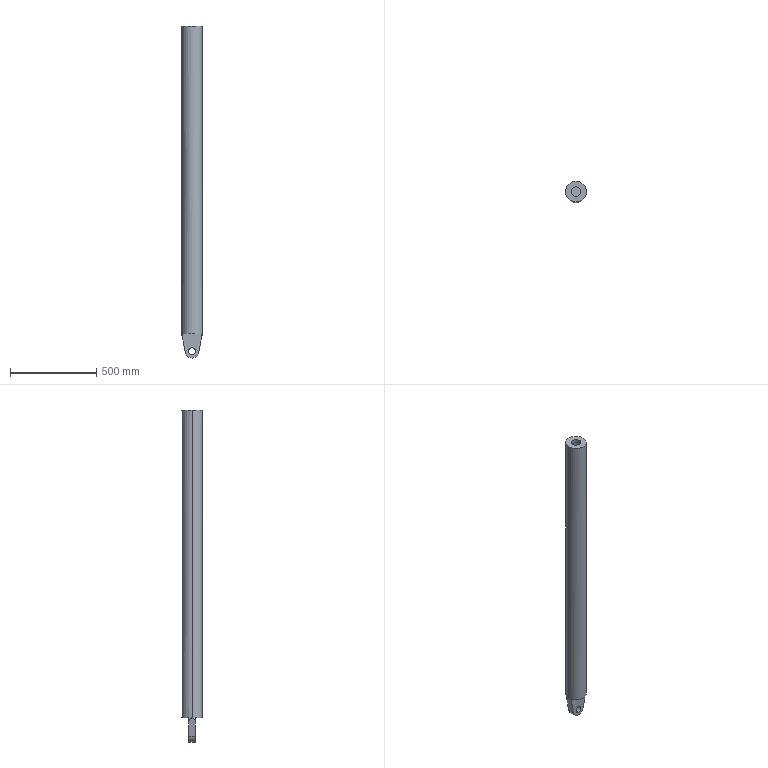Part | SolidWorks | features ICE 4, Extrusion 1 | 1 solid | 19 faces | box 120 x 120 x 1920 mm | volume 9594518 mm3 | cylinder 10 | plane 9 | commonest cylinder face diameters 40 x2 55 x2 80 x2 90 x2 120 x2
STEP:
#1=CARTESIAN_POINT('',(-45.,0.,1760.));
#2=VERTEX_POINT('',#1);
#3=CARTESIAN_POINT('',(45.,0.,1760.));
#4=VERTEX_POINT('',#3);
#5=CARTESIAN_POINT('',(0.,0.,1760.));
#6=DIRECTION('',(0.,0.,1.));
#7=DIRECTION('',(1.,0.,0.));
#8=AXIS2_PLACEMENT_3D('',#5,#6,#7);
#9=CIRCLE('',#8,45.);
#10=EDGE_CURVE('',#2,#4,#9,.T.);
#11=ORIENTED_EDGE('',*,*,#10,.T.);
#12=CARTESIAN_POINT('',(45.,0.,40.));
#13=VERTEX_POINT('',#12);
#14=CARTESIAN_POINT('',(45.,0.,1780.));
#15=DIRECTION('',(0.,0.,-1.));
#16=VECTOR('',#15,1000.);
#17=LINE('',#14,#16);
#18=EDGE_CURVE('',#4,#13,#17,.T.);
#19=ORIENTED_EDGE('',*,*,#18,.T.);
#20=CARTESIAN_POINT('',(-45.,0.,40.));
#21=VERTEX_POINT('',#20);
#22=CARTESIAN_POINT('',(0.,0.,40.));
#23=DIRECTION('',(0.,0.,-1.));
#24=DIRECTION('',(-1.,0.,0.));
#25=AXIS2_PLACEMENT_3D('',#22,#23,#24);
#26=CIRCLE('',#25,45.);
#27=EDGE_CURVE('',#13,#21,#26,.T.);
#28=ORIENTED_EDGE('',*,*,#27,.T.);
#29=CARTESIAN_POINT('',(-45.,0.,1780.));
#30=DIRECTION('',(0.,0.,-1.));
#31=VECTOR('',#30,1000.);
#32=LINE('',#29,#31);
#33=EDGE_CURVE('',#2,#21,#32,.T.);
#34=ORIENTED_EDGE('',*,*,#33,.F.);
#35=EDGE_LOOP('',(#11,#19,#28,#34));
#36=FACE_OUTER_BOUND('',#35,.T.);
#37=CARTESIAN_POINT('',(0.,0.,1780.));
#38=DIRECTION('',(0.,0.,-1.));
#39=DIRECTION('',(-1.,0.,0.));
#40=AXIS2_PLACEMENT_3D('',#37,#38,#39);
#41=CYLINDRICAL_SURFACE('',#40,45.);
#42=ADVANCED_FACE('',(#36),#41,.F.);
#43=CARTESIAN_POINT('',(-27.5,0.,1760.));
#44=VERTEX_POINT('',#43);
#45=CARTESIAN_POINT('',(27.5,0.,1760.));
#46=VERTEX_POINT('',#45);
#47=CARTESIAN_POINT('',(0.,0.,1760.));
#48=DIRECTION('',(0.,0.,1.));
#49=DIRECTION('',(1.,0.,0.));
#50=AXIS2_PLACEMENT_3D('',#47,#48,#49);
#51=CIRCLE('',#50,27.5);
#52=EDGE_CURVE('',#44,#46,#51,.T.);
#53=ORIENTED_EDGE('',*,*,#52,.F.);
#54=CARTESIAN_POINT('',(-27.5,0.,1780.));
#55=VERTEX_POINT('',#54);
#56=CARTESIAN_POINT('',(-27.5,0.,1760.));
#57=DIRECTION('',(0.,0.,1.));
#58=VECTOR('',#57,1000.);
#59=LINE('',#56,#58);
#60=EDGE_CURVE('',#44,#55,#59,.T.);
#61=ORIENTED_EDGE('',*,*,#60,.T.);
#62=CARTESIAN_POINT('',(27.5,0.,1780.));
#63=VERTEX_POINT('',#62);
#64=CARTESIAN_POINT('',(0.,0.,1780.));
#65=DIRECTION('',(0.,0.,1.));
#66=DIRECTION('',(1.,0.,0.));
#67=AXIS2_PLACEMENT_3D('',#64,#65,#66);
#68=CIRCLE('',#67,27.5);
#69=EDGE_CURVE('',#55,#63,#68,.T.);
#70=ORIENTED_EDGE('',*,*,#69,.T.);
#71=CARTESIAN_POINT('',(27.5,0.,1760.));
#72=DIRECTION('',(0.,0.,1.));
#73=VECTOR('',#72,1000.);
#74=LINE('',#71,#73);
#75=EDGE_CURVE('',#46,#63,#74,.T.);
#76=ORIENTED_EDGE('',*,*,#75,.F.);
#77=EDGE_LOOP('',(#53,#61,#70,#76));
#78=FACE_OUTER_BOUND('',#77,.T.);
#79=CARTESIAN_POINT('',(0.,0.,1760.));
#80=DIRECTION('',(0.,0.,1.));
#81=DIRECTION('',(1.,0.,0.));
#82=AXIS2_PLACEMENT_3D('',#79,#80,#81);
#83=CYLINDRICAL_SURFACE('',#82,27.5);
#84=ADVANCED_FACE('',(#78),#83,.F.);
#85=CARTESIAN_POINT('',(0.,20.,-120.));
#86=VERTEX_POINT('',#85);
#87=CARTESIAN_POINT('',(0.,20.,-80.));
#88=VERTEX_POINT('',#87);
#89=CARTESIAN_POINT('',(0.,20.,-100.));
#90=DIRECTION('',(0.,1.,0.));
#91=DIRECTION('',(0.,0.,1.));
#92=AXIS2_PLACEMENT_3D('',#89,#90,#91);
#93=CIRCLE('',#92,20.);
#94=EDGE_CURVE('',#86,#88,#93,.T.);
#95=ORIENTED_EDGE('',*,*,#94,.T.);
#96=CARTESIAN_POINT('',(0.,-20.,-80.));
#97=VERTEX_POINT('',#96);
#98=CARTESIAN_POINT('',(0.,20.,-80.));
#99=DIRECTION('',(0.,-1.,0.));
#100=VECTOR('',#99,1000.);
#101=LINE('',#98,#100);
#102=EDGE_CURVE('',#88,#97,#101,.T.);
#103=ORIENTED_EDGE('',*,*,#102,.T.);
#104=CARTESIAN_POINT('',(0.,-20.,-120.));
#105=VERTEX_POINT('',#104);
#106=CARTESIAN_POINT('',(0.,-20.,-100.));
#107=DIRECTION('',(0.,1.,0.));
#108=DIRECTION('',(0.,0.,1.));
#109=AXIS2_PLACEMENT_3D('',#106,#107,#108);
#110=CIRCLE('',#109,20.);
#111=EDGE_CURVE('',#105,#97,#110,.T.);
#112=ORIENTED_EDGE('',*,*,#111,.F.);
#113=CARTESIAN_POINT('',(0.,20.,-120.));
#114=DIRECTION('',(0.,-1.,0.));
#115=VECTOR('',#114,1000.);
#116=LINE('',#113,#115);
#117=EDGE_CURVE('',#86,#105,#116,.T.);
#118=ORIENTED_EDGE('',*,*,#117,.F.);
#119=EDGE_LOOP('',(#95,#103,#112,#118));
#120=FACE_OUTER_BOUND('',#119,.T.);
#121=CARTESIAN_POINT('',(0.,20.,-100.));
#122=DIRECTION('',(0.,-1.,0.));
#123=DIRECTION('',(0.,0.,-1.));
#124=AXIS2_PLACEMENT_3D('',#121,#122,#123);
#125=CYLINDRICAL_SURFACE('',#124,20.);
#126=ADVANCED_FACE('',(#120),#125,.F.);
#127=CARTESIAN_POINT('',(0.,20.,-140.));
#128=VERTEX_POINT('',#127);
#129=CARTESIAN_POINT('',(-39.278,20.,-107.567));
#130=VERTEX_POINT('',#129);
#131=CARTESIAN_POINT('',(0.,20.,-100.));
#132=DIRECTION('',(0.,1.,0.));
#133=DIRECTION('',(0.,0.,1.));
#134=AXIS2_PLACEMENT_3D('',#131,#132,#133);
#135=CIRCLE('',#134,40.);
#136=EDGE_CURVE('',#128,#130,#135,.T.);
#137=ORIENTED_EDGE('',*,*,#136,.F.);
#138=CARTESIAN_POINT('',(0.,-20.,-140.));
#139=VERTEX_POINT('',#138);
#140=CARTESIAN_POINT('',(0.,20.,-140.));
#141=DIRECTION('',(0.,-1.,0.));
#142=VECTOR('',#141,1000.);
#143=LINE('',#140,#142);
#144=EDGE_CURVE('',#128,#139,#143,.T.);
#145=ORIENTED_EDGE('',*,*,#144,.T.);
#146=CARTESIAN_POINT('',(-39.278,-20.,-107.567));
#147=VERTEX_POINT('',#146);
#148=CARTESIAN_POINT('',(0.,-20.,-100.));
#149=DIRECTION('',(0.,1.,0.));
#150=DIRECTION('',(0.,0.,1.));
#151=AXIS2_PLACEMENT_3D('',#148,#149,#150);
#152=CIRCLE('',#151,40.);
#153=EDGE_CURVE('',#139,#147,#152,.T.);
#154=ORIENTED_EDGE('',*,*,#153,.T.);
#155=CARTESIAN_POINT('',(-39.278,20.,-107.567));
#156=DIRECTION('',(0.,-1.,0.));
#157=VECTOR('',#156,1000.);
#158=LINE('',#155,#157);
#159=EDGE_CURVE('',#130,#147,#158,.T.);
#160=ORIENTED_EDGE('',*,*,#159,.F.);
#161=EDGE_LOOP('',(#137,#145,#154,#160));
#162=FACE_OUTER_BOUND('',#161,.T.);
#163=CARTESIAN_POINT('',(0.,20.,-100.));
#164=DIRECTION('',(0.,-1.,0.));
#165=DIRECTION('',(0.,0.,-1.));
#166=AXIS2_PLACEMENT_3D('',#163,#164,#165);
#167=CYLINDRICAL_SURFACE('',#166,40.);
#168=ADVANCED_FACE('',(#162),#167,.T.);
#169=CARTESIAN_POINT('',(60.,0.,1780.));
#170=VERTEX_POINT('',#169);
#171=CARTESIAN_POINT('',(-60.,0.,1780.));
#172=VERTEX_POINT('',#171);
#173=CARTESIAN_POINT('',(0.,0.,1780.));
#174=DIRECTION('',(0.,0.,1.));
#175=DIRECTION('',(1.,0.,0.));
#176=AXIS2_PLACEMENT_3D('',#173,#174,#175);
#177=CIRCLE('',#176,60.);
#178=EDGE_CURVE('',#170,#172,#177,.T.);
#179=ORIENTED_EDGE('',*,*,#178,.F.);
#180=CARTESIAN_POINT('',(60.,0.,0.));
#181=VERTEX_POINT('',#180);
#182=CARTESIAN_POINT('',(60.,0.,1780.));
#183=DIRECTION('',(0.,0.,-1.));
#184=VECTOR('',#183,1000.);
#185=LINE('',#182,#184);
#186=EDGE_CURVE('',#170,#181,#185,.T.);
#187=ORIENTED_EDGE('',*,*,#186,.T.);
#188=CARTESIAN_POINT('',(56.569,20.,-17.812));
#189=VERTEX_POINT('',#188);
#190=CARTESIAN_POINT('',(56.569,20.,-17.812));
#191=CARTESIAN_POINT('',(58.845,13.561,-5.995));
#192=CARTESIAN_POINT('',(60.,6.83,0.));
#193=CARTESIAN_POINT('',(60.,0.,0.));
#194=(BOUNDED_CURVE()B_SPLINE_CURVE(3,(#190,#191,#192,#193),.UNSPECIFIED.,.F.,.F.)B_SPLINE_CURVE_WITH_KNOTS((4,4),(5.943,6.283),.UNSPECIFIED.)CURVE()GEOMETRIC_REPRESENTATION_ITEM()RATIONAL_B_SPLINE_CURVE((1.,0.9904,0.9904,1.))REPRESENTATION_ITEM(''));
#195=EDGE_CURVE('',#189,#181,#194,.T.);
#196=ORIENTED_EDGE('',*,*,#195,.F.);
#197=CARTESIAN_POINT('',(56.569,20.,0.));
#198=VERTEX_POINT('',#197);
#199=CARTESIAN_POINT('',(56.569,20.,-140.));
#200=DIRECTION('',(0.,0.,1.));
#201=VECTOR('',#200,1000.);
#202=LINE('',#199,#201);
#203=EDGE_CURVE('',#189,#198,#202,.T.);
#204=ORIENTED_EDGE('',*,*,#203,.T.);
#205=CARTESIAN_POINT('',(-56.569,20.,0.));
#206=VERTEX_POINT('',#205);
#207=CARTESIAN_POINT('',(0.,0.,0.));
#208=DIRECTION('',(0.,0.,1.));
#209=DIRECTION('',(1.,0.,0.));
#210=AXIS2_PLACEMENT_3D('',#207,#208,#209);
#211=CIRCLE('',#210,60.);
#212=EDGE_CURVE('',#198,#206,#211,.T.);
#213=ORIENTED_EDGE('',*,*,#212,.T.);
#214=CARTESIAN_POINT('',(-56.569,20.,-17.812));
#215=VERTEX_POINT('',#214);
#216=CARTESIAN_POINT('',(-56.569,20.,-140.));
#217=DIRECTION('',(0.,0.,-1.));
#218=VECTOR('',#217,1000.);
#219=LINE('',#216,#218);
#220=EDGE_CURVE('',#206,#215,#219,.T.);
#221=ORIENTED_EDGE('',*,*,#220,.T.);
#222=CARTESIAN_POINT('',(-60.,0.,0.));
#223=VERTEX_POINT('',#222);
#224=CARTESIAN_POINT('',(-60.,0.,0.));
#225=CARTESIAN_POINT('',(-60.,6.83,0.));
#226=CARTESIAN_POINT('',(-58.845,13.561,-5.995));
#227=CARTESIAN_POINT('',(-56.569,20.,-17.812));
#228=(BOUNDED_CURVE()B_SPLINE_CURVE(3,(#224,#225,#226,#227),.UNSPECIFIED.,.F.,.F.)B_SPLINE_CURVE_WITH_KNOTS((4,4),(0.,0.3398),.UNSPECIFIED.)CURVE()GEOMETRIC_REPRESENTATION_ITEM()RATIONAL_B_SPLINE_CURVE((1.,0.9904,0.9904,1.))REPRESENTATION_ITEM(''));
#229=EDGE_CURVE('',#223,#215,#228,.T.);
#230=ORIENTED_EDGE('',*,*,#229,.F.);
#231=CARTESIAN_POINT('',(-60.,0.,1780.));
#232=DIRECTION('',(0.,0.,-1.));
#233=VECTOR('',#232,1000.);
#234=LINE('',#231,#233);
#235=EDGE_CURVE('',#172,#223,#234,.T.);
#236=ORIENTED_EDGE('',*,*,#235,.F.);
#237=EDGE_LOOP('',(#179,#187,#196,#204,#213,#221,#230,#236));
#238=FACE_OUTER_BOUND('',#237,.T.);
#239=CARTESIAN_POINT('',(0.,0.,1780.));
#240=DIRECTION('',(0.,0.,-1.));
#241=DIRECTION('',(-1.,0.,0.));
#242=AXIS2_PLACEMENT_3D('',#239,#240,#241);
#243=CYLINDRICAL_SURFACE('',#242,60.);
#244=ADVANCED_FACE('',(#238),#243,.T.);
#245=CARTESIAN_POINT('',(39.278,20.,-107.567));
#246=VERTEX_POINT('',#245);
#247=CARTESIAN_POINT('',(60.,20.,0.));
#248=DIRECTION('',(-0.1892,0.,-0.9819));
#249=VECTOR('',#248,1000.);
#250=LINE('',#247,#249);
#251=EDGE_CURVE('',#189,#246,#250,.T.);
#252=ORIENTED_EDGE('',*,*,#251,.F.);
#253=ORIENTED_EDGE('',*,*,#195,.T.);
#254=CARTESIAN_POINT('',(56.569,-20.,-17.812));
#255=VERTEX_POINT('',#254);
#256=CARTESIAN_POINT('',(60.,0.,0.));
#257=CARTESIAN_POINT('',(60.,-6.83,0.));
#258=CARTESIAN_POINT('',(58.845,-13.561,-5.995));
#259=CARTESIAN_POINT('',(56.569,-20.,-17.812));
#260=(BOUNDED_CURVE()B_SPLINE_CURVE(3,(#256,#257,#258,#259),.UNSPECIFIED.,.F.,.F.)B_SPLINE_CURVE_WITH_KNOTS((4,4),(0.,0.3398),.UNSPECIFIED.)CURVE()GEOMETRIC_REPRESENTATION_ITEM()RATIONAL_B_SPLINE_CURVE((1.,0.9904,0.9904,1.))REPRESENTATION_ITEM(''));
#261=EDGE_CURVE('',#181,#255,#260,.T.);
#262=ORIENTED_EDGE('',*,*,#261,.T.);
#263=CARTESIAN_POINT('',(39.278,-20.,-107.567));
#264=VERTEX_POINT('',#263);
#265=CARTESIAN_POINT('',(60.,-20.,0.));
#266=DIRECTION('',(-0.1892,0.,-0.9819));
#267=VECTOR('',#266,1000.);
#268=LINE('',#265,#267);
#269=EDGE_CURVE('',#255,#264,#268,.T.);
#270=ORIENTED_EDGE('',*,*,#269,.T.);
#271=CARTESIAN_POINT('',(39.278,20.,-107.567));
#272=DIRECTION('',(0.,-1.,0.));
#273=VECTOR('',#272,1000.);
#274=LINE('',#271,#273);
#275=EDGE_CURVE('',#246,#264,#274,.T.);
#276=ORIENTED_EDGE('',*,*,#275,.F.);
#277=EDGE_LOOP('',(#252,#253,#262,#270,#276));
#278=FACE_OUTER_BOUND('',#277,.T.);
#279=CARTESIAN_POINT('',(60.,20.,0.));
#280=DIRECTION('',(-0.9819,0.,0.1892));
#281=DIRECTION('',(0.1892,0.,0.9819));
#282=AXIS2_PLACEMENT_3D('',#279,#280,#281);
#283=PLANE('',#282);
#284=ADVANCED_FACE('',(#278),#283,.F.);
#285=CARTESIAN_POINT('',(-56.569,-20.,-17.812));
#286=VERTEX_POINT('',#285);
#287=CARTESIAN_POINT('',(-56.569,-20.,-17.812));
#288=CARTESIAN_POINT('',(-58.845,-13.561,-5.995));
#289=CARTESIAN_POINT('',(-60.,-6.83,0.));
#290=CARTESIAN_POINT('',(-60.,0.,0.));
#291=(BOUNDED_CURVE()B_SPLINE_CURVE(3,(#287,#288,#289,#290),.UNSPECIFIED.,.F.,.F.)B_SPLINE_CURVE_WITH_KNOTS((4,4),(5.943,6.283),.UNSPECIFIED.)CURVE()GEOMETRIC_REPRESENTATION_ITEM()RATIONAL_B_SPLINE_CURVE((1.,0.9904,0.9904,1.))REPRESENTATION_ITEM(''));
#292=EDGE_CURVE('',#286,#223,#291,.T.);
#293=ORIENTED_EDGE('',*,*,#292,.T.);
#294=ORIENTED_EDGE('',*,*,#229,.T.);
#295=CARTESIAN_POINT('',(-60.,20.,0.));
#296=DIRECTION('',(-0.1892,0.,0.9819));
#297=VECTOR('',#296,1000.);
#298=LINE('',#295,#297);
#299=EDGE_CURVE('',#130,#215,#298,.T.);
#300=ORIENTED_EDGE('',*,*,#299,.F.);
#301=ORIENTED_EDGE('',*,*,#159,.T.);
#302=CARTESIAN_POINT('',(-60.,-20.,0.));
#303=DIRECTION('',(-0.1892,0.,0.9819));
#304=VECTOR('',#303,1000.);
#305=LINE('',#302,#304);
#306=EDGE_CURVE('',#147,#286,#305,.T.);
#307=ORIENTED_EDGE('',*,*,#306,.T.);
#308=EDGE_LOOP('',(#293,#294,#300,#301,#307));
#309=FACE_OUTER_BOUND('',#308,.T.);
#310=CARTESIAN_POINT('',(-60.,20.,0.));
#311=DIRECTION('',(0.9819,0.,0.1892));
#312=DIRECTION('',(0.1892,0.,-0.9819));
#313=AXIS2_PLACEMENT_3D('',#310,#311,#312);
#314=PLANE('',#313);
#315=ADVANCED_FACE('',(#309),#314,.F.);
#316=ORIENTED_EDGE('',*,*,#212,.F.);
#317=CARTESIAN_POINT('',(-60.,20.,0.));
#318=DIRECTION('',(1.,0.,0.));
#319=VECTOR('',#318,1000.);
#320=LINE('',#317,#319);
#321=EDGE_CURVE('',#206,#198,#320,.T.);
#322=ORIENTED_EDGE('',*,*,#321,.F.);
#323=EDGE_LOOP('',(#316,#322));
#324=FACE_OUTER_BOUND('',#323,.T.);
#325=CARTESIAN_POINT('',(0.,0.,0.));
#326=DIRECTION('',(0.,0.,1.));
#327=DIRECTION('',(1.,0.,0.));
#328=AXIS2_PLACEMENT_3D('',#325,#326,#327);
#329=PLANE('',#328);
#330=ADVANCED_FACE('',(#324),#329,.F.);
#331=CARTESIAN_POINT('',(0.,0.,1780.));
#332=DIRECTION('',(0.,0.,1.));
#333=DIRECTION('',(1.,0.,0.));
#334=AXIS2_PLACEMENT_3D('',#331,#332,#333);
#335=CIRCLE('',#334,60.);
#336=EDGE_CURVE('',#172,#170,#335,.T.);
#337=ORIENTED_EDGE('',*,*,#336,.T.);
#338=ORIENTED_EDGE('',*,*,#178,.T.);
#339=EDGE_LOOP('',(#337,#338));
#340=FACE_OUTER_BOUND('',#339,.T.);
#341=CARTESIAN_POINT('',(0.,0.,1780.));
#342=DIRECTION('',(0.,0.,1.));
#343=DIRECTION('',(1.,0.,0.));
#344=AXIS2_PLACEMENT_3D('',#341,#342,#343);
#345=CIRCLE('',#344,27.5);
#346=EDGE_CURVE('',#63,#55,#345,.T.);
#347=ORIENTED_EDGE('',*,*,#346,.F.);
#348=ORIENTED_EDGE('',*,*,#69,.F.);
#349=EDGE_LOOP('',(#347,#348));
#350=FACE_BOUND('',#349,.T.);
#351=CARTESIAN_POINT('',(0.,0.,1780.));
#352=DIRECTION('',(0.,0.,1.));
#353=DIRECTION('',(1.,0.,0.));
#354=AXIS2_PLACEMENT_3D('',#351,#352,#353);
#355=PLANE('',#354);
#356=ADVANCED_FACE('',(#340,#350),#355,.T.);
#357=CARTESIAN_POINT('',(-56.569,-20.,0.));
#358=VERTEX_POINT('',#357);
#359=CARTESIAN_POINT('',(56.569,-20.,0.));
#360=VERTEX_POINT('',#359);
#361=CARTESIAN_POINT('',(0.,0.,0.));
#362=DIRECTION('',(0.,0.,1.));
#363=DIRECTION('',(1.,0.,0.));
#364=AXIS2_PLACEMENT_3D('',#361,#362,#363);
#365=CIRCLE('',#364,60.);
#366=EDGE_CURVE('',#358,#360,#365,.T.);
#367=ORIENTED_EDGE('',*,*,#366,.F.);
#368=CARTESIAN_POINT('',(-60.,-20.,0.));
#369=DIRECTION('',(1.,0.,0.));
#370=VECTOR('',#369,1000.);
#371=LINE('',#368,#370);
#372=EDGE_CURVE('',#358,#360,#371,.T.);
#373=ORIENTED_EDGE('',*,*,#372,.T.);
#374=EDGE_LOOP('',(#367,#373));
#375=FACE_OUTER_BOUND('',#374,.T.);
#376=CARTESIAN_POINT('',(0.,0.,0.));
#377=DIRECTION('',(0.,0.,1.));
#378=DIRECTION('',(1.,0.,0.));
#379=AXIS2_PLACEMENT_3D('',#376,#377,#378);
#380=PLANE('',#379);
#381=ADVANCED_FACE('',(#375),#380,.F.);
#382=ORIENTED_EDGE('',*,*,#186,.F.);
#383=ORIENTED_EDGE('',*,*,#336,.F.);
#384=ORIENTED_EDGE('',*,*,#235,.T.);
#385=ORIENTED_EDGE('',*,*,#292,.F.);
#386=CARTESIAN_POINT('',(-56.569,-20.,-140.));
#387=DIRECTION('',(0.,0.,-1.));
#388=VECTOR('',#387,1000.);
#389=LINE('',#386,#388);
#390=EDGE_CURVE('',#358,#286,#389,.T.);
#391=ORIENTED_EDGE('',*,*,#390,.F.);
#392=ORIENTED_EDGE('',*,*,#366,.T.);
#393=CARTESIAN_POINT('',(56.569,-20.,-140.));
#394=DIRECTION('',(0.,0.,1.));
#395=VECTOR('',#394,1000.);
#396=LINE('',#393,#395);
#397=EDGE_CURVE('',#255,#360,#396,.T.);
#398=ORIENTED_EDGE('',*,*,#397,.F.);
#399=ORIENTED_EDGE('',*,*,#261,.F.);
#400=EDGE_LOOP('',(#382,#383,#384,#385,#391,#392,#398,#399));
#401=FACE_OUTER_BOUND('',#400,.T.);
#402=CARTESIAN_POINT('',(0.,0.,1780.));
#403=DIRECTION('',(0.,0.,-1.));
#404=DIRECTION('',(-1.,0.,0.));
#405=AXIS2_PLACEMENT_3D('',#402,#403,#404);
#406=CYLINDRICAL_SURFACE('',#405,60.);
#407=ADVANCED_FACE('',(#401),#406,.T.);
#408=ORIENTED_EDGE('',*,*,#220,.F.);
#409=ORIENTED_EDGE('',*,*,#321,.T.);
#410=ORIENTED_EDGE('',*,*,#203,.F.);
#411=ORIENTED_EDGE('',*,*,#251,.T.);
#412=CARTESIAN_POINT('',(0.,20.,-100.));
#413=DIRECTION('',(0.,1.,0.));
#414=DIRECTION('',(0.,0.,1.));
#415=AXIS2_PLACEMENT_3D('',#412,#413,#414);
#416=CIRCLE('',#415,40.);
#417=EDGE_CURVE('',#246,#128,#416,.T.);
#418=ORIENTED_EDGE('',*,*,#417,.T.);
#419=ORIENTED_EDGE('',*,*,#136,.T.);
#420=ORIENTED_EDGE('',*,*,#299,.T.);
#421=EDGE_LOOP('',(#408,#409,#410,#411,#418,#419,#420));
#422=FACE_OUTER_BOUND('',#421,.T.);
#423=ORIENTED_EDGE('',*,*,#94,.F.);
#424=CARTESIAN_POINT('',(0.,20.,-100.));
#425=DIRECTION('',(0.,1.,0.));
#426=DIRECTION('',(0.,0.,1.));
#427=AXIS2_PLACEMENT_3D('',#424,#425,#426);
#428=CIRCLE('',#427,20.);
#429=EDGE_CURVE('',#88,#86,#428,.T.);
#430=ORIENTED_EDGE('',*,*,#429,.F.);
#431=EDGE_LOOP('',(#423,#430));
#432=FACE_BOUND('',#431,.T.);
#433=CARTESIAN_POINT('',(0.,20.,-100.));
#434=DIRECTION('',(0.,1.,0.));
#435=DIRECTION('',(0.,0.,1.));
#436=AXIS2_PLACEMENT_3D('',#433,#434,#435);
#437=PLANE('',#436);
#438=ADVANCED_FACE('',(#422,#432),#437,.T.);
#439=ORIENTED_EDGE('',*,*,#372,.F.);
#440=ORIENTED_EDGE('',*,*,#390,.T.);
#441=ORIENTED_EDGE('',*,*,#306,.F.);
#442=ORIENTED_EDGE('',*,*,#153,.F.);
#443=CARTESIAN_POINT('',(0.,-20.,-100.));
#444=DIRECTION('',(0.,1.,0.));
#445=DIRECTION('',(0.,0.,1.));
#446=AXIS2_PLACEMENT_3D('',#443,#444,#445);
#447=CIRCLE('',#446,40.);
#448=EDGE_CURVE('',#264,#139,#447,.T.);
#449=ORIENTED_EDGE('',*,*,#448,.F.);
#450=ORIENTED_EDGE('',*,*,#269,.F.);
#451=ORIENTED_EDGE('',*,*,#397,.T.);
#452=EDGE_LOOP('',(#439,#440,#441,#442,#449,#450,#451));
#453=FACE_OUTER_BOUND('',#452,.T.);
#454=ORIENTED_EDGE('',*,*,#111,.T.);
#455=CARTESIAN_POINT('',(0.,-20.,-100.));
#456=DIRECTION('',(0.,1.,0.));
#457=DIRECTION('',(0.,0.,1.));
#458=AXIS2_PLACEMENT_3D('',#455,#456,#457);
#459=CIRCLE('',#458,20.);
#460=EDGE_CURVE('',#97,#105,#459,.T.);
#461=ORIENTED_EDGE('',*,*,#460,.T.);
#462=EDGE_LOOP('',(#454,#461));
#463=FACE_BOUND('',#462,.T.);
#464=CARTESIAN_POINT('',(0.,-20.,-100.));
#465=DIRECTION('',(0.,1.,0.));
#466=DIRECTION('',(0.,0.,1.));
#467=AXIS2_PLACEMENT_3D('',#464,#465,#466);
#468=PLANE('',#467);
#469=ADVANCED_FACE('',(#453,#463),#468,.F.);
#470=ORIENTED_EDGE('',*,*,#144,.F.);
#471=ORIENTED_EDGE('',*,*,#417,.F.);
#472=ORIENTED_EDGE('',*,*,#275,.T.);
#473=ORIENTED_EDGE('',*,*,#448,.T.);
#474=EDGE_LOOP('',(#470,#471,#472,#473));
#475=FACE_OUTER_BOUND('',#474,.T.);
#476=CARTESIAN_POINT('',(0.,20.,-100.));
#477=DIRECTION('',(0.,-1.,0.));
#478=DIRECTION('',(0.,0.,-1.));
#479=AXIS2_PLACEMENT_3D('',#476,#477,#478);
#480=CYLINDRICAL_SURFACE('',#479,40.);
#481=ADVANCED_FACE('',(#475),#480,.T.);
#482=ORIENTED_EDGE('',*,*,#102,.F.);
#483=ORIENTED_EDGE('',*,*,#429,.T.);
#484=ORIENTED_EDGE('',*,*,#117,.T.);
#485=ORIENTED_EDGE('',*,*,#460,.F.);
#486=EDGE_LOOP('',(#482,#483,#484,#485));
#487=FACE_OUTER_BOUND('',#486,.T.);
#488=CARTESIAN_POINT('',(0.,20.,-100.));
#489=DIRECTION('',(0.,-1.,0.));
#490=DIRECTION('',(0.,0.,-1.));
#491=AXIS2_PLACEMENT_3D('',#488,#489,#490);
#492=CYLINDRICAL_SURFACE('',#491,20.);
#493=ADVANCED_FACE('',(#487),#492,.F.);
#494=ORIENTED_EDGE('',*,*,#10,.F.);
#495=CARTESIAN_POINT('',(0.,0.,1760.));
#496=DIRECTION('',(0.,0.,1.));
#497=DIRECTION('',(1.,0.,0.));
#498=AXIS2_PLACEMENT_3D('',#495,#496,#497);
#499=CIRCLE('',#498,45.);
#500=EDGE_CURVE('',#4,#2,#499,.T.);
#501=ORIENTED_EDGE('',*,*,#500,.F.);
#502=EDGE_LOOP('',(#494,#501));
#503=FACE_OUTER_BOUND('',#502,.T.);
#504=CARTESIAN_POINT('',(0.,0.,1760.));
#505=DIRECTION('',(0.,0.,1.));
#506=DIRECTION('',(1.,0.,0.));
#507=AXIS2_PLACEMENT_3D('',#504,#505,#506);
#508=CIRCLE('',#507,27.5);
#509=EDGE_CURVE('',#46,#44,#508,.T.);
#510=ORIENTED_EDGE('',*,*,#509,.T.);
#511=ORIENTED_EDGE('',*,*,#52,.T.);
#512=EDGE_LOOP('',(#510,#511));
#513=FACE_BOUND('',#512,.T.);
#514=CARTESIAN_POINT('',(0.,0.,1760.));
#515=DIRECTION('',(0.,0.,1.));
#516=DIRECTION('',(1.,0.,0.));
#517=AXIS2_PLACEMENT_3D('',#514,#515,#516);
#518=PLANE('',#517);
#519=ADVANCED_FACE('',(#503,#513),#518,.F.);
#520=ORIENTED_EDGE('',*,*,#60,.F.);
#521=ORIENTED_EDGE('',*,*,#509,.F.);
#522=ORIENTED_EDGE('',*,*,#75,.T.);
#523=ORIENTED_EDGE('',*,*,#346,.T.);
#524=EDGE_LOOP('',(#520,#521,#522,#523));
#525=FACE_OUTER_BOUND('',#524,.T.);
#526=CARTESIAN_POINT('',(0.,0.,1760.));
#527=DIRECTION('',(0.,0.,1.));
#528=DIRECTION('',(1.,0.,0.));
#529=AXIS2_PLACEMENT_3D('',#526,#527,#528);
#530=CYLINDRICAL_SURFACE('',#529,27.5);
#531=ADVANCED_FACE('',(#525),#530,.F.);
#532=CARTESIAN_POINT('',(0.,0.,40.));
#533=DIRECTION('',(0.,0.,-1.));
#534=DIRECTION('',(-1.,0.,0.));
#535=AXIS2_PLACEMENT_3D('',#532,#533,#534);
#536=CIRCLE('',#535,45.);
#537=EDGE_CURVE('',#21,#13,#536,.T.);
#538=ORIENTED_EDGE('',*,*,#537,.F.);
#539=ORIENTED_EDGE('',*,*,#27,.F.);
#540=EDGE_LOOP('',(#538,#539));
#541=FACE_OUTER_BOUND('',#540,.T.);
#542=CARTESIAN_POINT('',(0.,0.,40.));
#543=DIRECTION('',(0.,0.,-1.));
#544=DIRECTION('',(-1.,0.,0.));
#545=AXIS2_PLACEMENT_3D('',#542,#543,#544);
#546=PLANE('',#545);
#547=ADVANCED_FACE('',(#541),#546,.F.);
#548=ORIENTED_EDGE('',*,*,#18,.F.);
#549=ORIENTED_EDGE('',*,*,#500,.T.);
#550=ORIENTED_EDGE('',*,*,#33,.T.);
#551=ORIENTED_EDGE('',*,*,#537,.T.);
#552=EDGE_LOOP('',(#548,#549,#550,#551));
#553=FACE_OUTER_BOUND('',#552,.T.);
#554=CARTESIAN_POINT('',(0.,0.,1780.));
#555=DIRECTION('',(0.,0.,-1.));
#556=DIRECTION('',(-1.,0.,0.));
#557=AXIS2_PLACEMENT_3D('',#554,#555,#556);
#558=CYLINDRICAL_SURFACE('',#557,45.);
#559=ADVANCED_FACE('',(#553),#558,.F.);
#560=CLOSED_SHELL('',(#42,#84,#126,#168,#244,#284,#315,#330,#356,#381,#407,#438,#469,#481,#493,#519,#531,#547,#559));
#561=MANIFOLD_SOLID_BREP('',#560);
#562=CARTESIAN_POINT('',(0.,0.,0.));
#563=DIRECTION('',(0.,0.,1.));
#564=DIRECTION('',(1.,0.,0.));
#565=AXIS2_PLACEMENT_3D('',#562,#563,#564);
#566=(LENGTH_UNIT()NAMED_UNIT(*)SI_UNIT(.MILLI.,.METRE.));
#567=UNCERTAINTY_MEASURE_WITH_UNIT(LENGTH_MEASURE(0.00001),#566,'','');
#568=(NAMED_UNIT(*)PLANE_ANGLE_UNIT()SI_UNIT($,.RADIAN.));
#569=(NAMED_UNIT(*)SI_UNIT($,.STERADIAN.)SOLID_ANGLE_UNIT());
#570=(GEOMETRIC_REPRESENTATION_CONTEXT(3)GLOBAL_UNCERTAINTY_ASSIGNED_CONTEXT((#567))GLOBAL_UNIT_ASSIGNED_CONTEXT((#566,#568,#569))REPRESENTATION_CONTEXT('',''));
#571=ADVANCED_BREP_SHAPE_REPRESENTATION('',(#561,#565),#570);